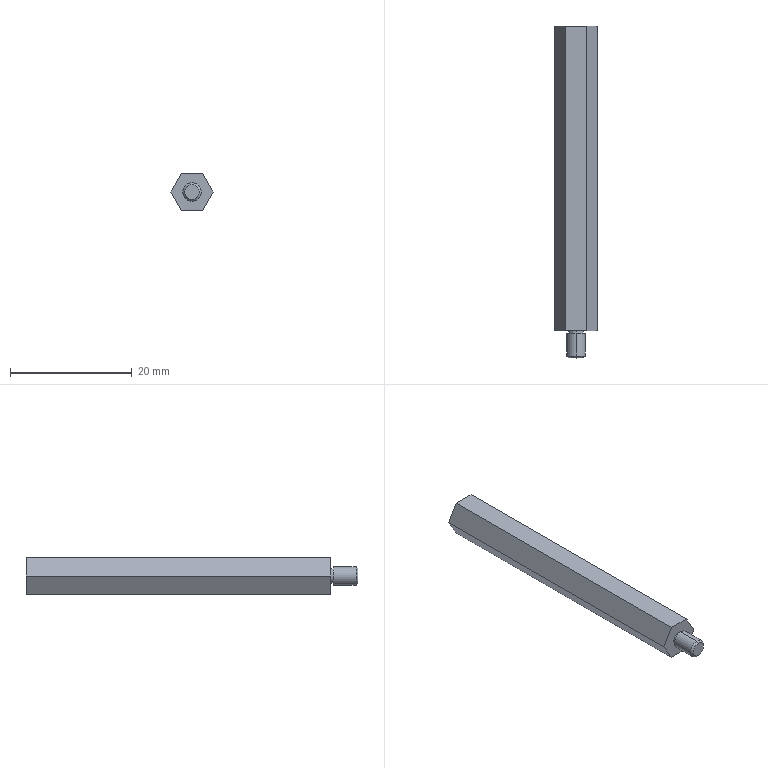Part | STEP file | 0230_017_LSBWRK6-50 | 1 solid | 22 faces | box 6.928 x 54.5 x 6 mm | volume 1554 mm3 | plane 10 | cone 6 | cylinder 6 | commonest cylinder face diameters 2.4 x2 2.5 x2 3 x2
STEP:
#1=CARTESIAN_POINT('',(0.,0.,0.));
#2=DIRECTION('',(0.,0.,1.));
#3=DIRECTION('',(1.,0.,0.));
#4=AXIS2_PLACEMENT_3D('',#1,#2,#3);
#5=CARTESIAN_POINT('',(0.,49.844,1.25));
#6=VERTEX_POINT('',#5);
#7=CARTESIAN_POINT('',(0.,50.,1.52));
#8=VERTEX_POINT('',#7);
#9=CARTESIAN_POINT('',(0.,49.844,1.25));
#10=DIRECTION('',(0.,0.5,0.866));
#11=VECTOR('',#10,1.);
#12=LINE('',#9,#11);
#13=CARTESIAN_POINT('',(0.,49.844,0.));
#14=DIRECTION('',(0.,1.,0.));
#15=DIRECTION('',(0.,0.,1.));
#16=AXIS2_PLACEMENT_3D('',#13,#14,#15);
#17=CONICAL_SURFACE('',#16,1.25,1.047);
#18=CARTESIAN_POINT('',(6.283,0.));
#19=DIRECTION('',(0.,1.));
#20=VECTOR('',#19,1.);
#21=LINE('',#18,#20);
#22=(GEOMETRIC_REPRESENTATION_CONTEXT(2)PARAMETRIC_REPRESENTATION_CONTEXT()REPRESENTATION_CONTEXT('',''));
#23=DEFINITIONAL_REPRESENTATION('',(#21),#22);
#24=PCURVE('',#17,#23);
#25=CARTESIAN_POINT('',(0.,49.844,0.));
#26=DIRECTION('',(0.,1.,0.));
#27=DIRECTION('',(0.,0.,1.));
#28=AXIS2_PLACEMENT_3D('',#25,#26,#27);
#29=CONICAL_SURFACE('',#28,1.25,1.047);
#30=CARTESIAN_POINT('',(0.,0.));
#31=DIRECTION('',(0.,1.));
#32=VECTOR('',#31,1.);
#33=LINE('',#30,#32);
#34=(GEOMETRIC_REPRESENTATION_CONTEXT(2)PARAMETRIC_REPRESENTATION_CONTEXT()REPRESENTATION_CONTEXT('',''));
#35=DEFINITIONAL_REPRESENTATION('',(#33),#34);
#36=PCURVE('',#29,#35);
#37=SURFACE_CURVE('',#12,(#24,#36),.PCURVE_S1.);
#38=EDGE_CURVE('',#6,#8,#37,.T.);
#39=ORIENTED_EDGE('',*,*,#38,.T.);
#40=CARTESIAN_POINT('',(0.,50.,-1.52));
#41=VERTEX_POINT('',#40);
#42=CARTESIAN_POINT('',(0.,50.,0.));
#43=DIRECTION('',(0.,-1.,0.));
#44=DIRECTION('',(1.,0.,0.));
#45=AXIS2_PLACEMENT_3D('',#42,#43,#44);
#46=CIRCLE('',#45,1.52);
#47=CARTESIAN_POINT('',(7.854,0.1559));
#48=DIRECTION('',(-1.,0.));
#49=VECTOR('',#48,1.);
#50=LINE('',#47,#49);
#51=(GEOMETRIC_REPRESENTATION_CONTEXT(2)PARAMETRIC_REPRESENTATION_CONTEXT()REPRESENTATION_CONTEXT('',''));
#52=DEFINITIONAL_REPRESENTATION('',(#50),#51);
#53=PCURVE('',#17,#52);
#54=CARTESIAN_POINT('',(3.464,50.,0.));
#55=DIRECTION('',(0.,-1.,0.));
#56=DIRECTION('',(1.,0.,0.));
#57=AXIS2_PLACEMENT_3D('',#54,#55,#56);
#58=PLANE('',#57);
#59=CARTESIAN_POINT('',(-3.464,0.));
#60=DIRECTION('',(1.,0.));
#61=AXIS2_PLACEMENT_2D('',#59,#60);
#62=CIRCLE('',#61,1.52);
#63=(GEOMETRIC_REPRESENTATION_CONTEXT(2)PARAMETRIC_REPRESENTATION_CONTEXT()REPRESENTATION_CONTEXT('',''));
#64=DEFINITIONAL_REPRESENTATION('',(#62),#63);
#65=PCURVE('',#58,#64);
#66=SURFACE_CURVE('',#46,(#53,#65),.PCURVE_S1.);
#67=EDGE_CURVE('',#8,#41,#66,.T.);
#68=ORIENTED_EDGE('',*,*,#67,.T.);
#69=CARTESIAN_POINT('',(0.,49.844,-1.25));
#70=VERTEX_POINT('',#69);
#71=CARTESIAN_POINT('',(0.,49.844,-1.25));
#72=DIRECTION('',(0.,0.5,-0.866));
#73=VECTOR('',#72,1.);
#74=LINE('',#71,#73);
#75=CARTESIAN_POINT('',(3.142,0.));
#76=DIRECTION('',(0.,1.));
#77=VECTOR('',#76,1.);
#78=LINE('',#75,#77);
#79=(GEOMETRIC_REPRESENTATION_CONTEXT(2)PARAMETRIC_REPRESENTATION_CONTEXT()REPRESENTATION_CONTEXT('',''));
#80=DEFINITIONAL_REPRESENTATION('',(#78),#79);
#81=PCURVE('',#17,#80);
#82=CARTESIAN_POINT('',(3.142,0.));
#83=DIRECTION('',(0.,1.));
#84=VECTOR('',#83,1.);
#85=LINE('',#82,#84);
#86=(GEOMETRIC_REPRESENTATION_CONTEXT(2)PARAMETRIC_REPRESENTATION_CONTEXT()REPRESENTATION_CONTEXT('',''));
#87=DEFINITIONAL_REPRESENTATION('',(#85),#86);
#88=PCURVE('',#29,#87);
#89=SURFACE_CURVE('',#74,(#81,#88),.PCURVE_S1.);
#90=EDGE_CURVE('',#70,#41,#89,.T.);
#91=ORIENTED_EDGE('',*,*,#90,.F.);
#92=CARTESIAN_POINT('',(0.,49.844,0.));
#93=DIRECTION('',(0.,1.,0.));
#94=DIRECTION('',(0.,0.,-1.));
#95=AXIS2_PLACEMENT_3D('',#92,#93,#94);
#96=CIRCLE('',#95,1.25);
#97=CARTESIAN_POINT('',(3.142,0.));
#98=DIRECTION('',(1.,0.));
#99=VECTOR('',#98,1.);
#100=LINE('',#97,#99);
#101=(GEOMETRIC_REPRESENTATION_CONTEXT(2)PARAMETRIC_REPRESENTATION_CONTEXT()REPRESENTATION_CONTEXT('',''));
#102=DEFINITIONAL_REPRESENTATION('',(#100),#101);
#103=PCURVE('',#17,#102);
#104=CARTESIAN_POINT('',(0.,50.,0.));
#105=DIRECTION('',(0.,1.,0.));
#106=DIRECTION('',(0.,0.,1.));
#107=AXIS2_PLACEMENT_3D('',#104,#105,#106);
#108=CYLINDRICAL_SURFACE('',#107,1.25);
#109=CARTESIAN_POINT('',(3.142,-0.1559));
#110=DIRECTION('',(1.,0.));
#111=VECTOR('',#110,1.);
#112=LINE('',#109,#111);
#113=(GEOMETRIC_REPRESENTATION_CONTEXT(2)PARAMETRIC_REPRESENTATION_CONTEXT()REPRESENTATION_CONTEXT('',''));
#114=DEFINITIONAL_REPRESENTATION('',(#112),#113);
#115=PCURVE('',#108,#114);
#116=SURFACE_CURVE('',#96,(#103,#115),.PCURVE_S1.);
#117=EDGE_CURVE('',#70,#6,#116,.T.);
#118=ORIENTED_EDGE('',*,*,#117,.T.);
#119=EDGE_LOOP('',(#39,#68,#91,#118));
#120=FACE_BOUND('',#119,.F.);
#121=ADVANCED_FACE('',(#120),#17,.F.);
#122=CARTESIAN_POINT('',(0.,-4.5,-1.193));
#123=VERTEX_POINT('',#122);
#124=CARTESIAN_POINT('',(0.,-4.5,1.193));
#125=VERTEX_POINT('',#124);
#126=CARTESIAN_POINT('',(0.,-4.5,0.));
#127=DIRECTION('',(0.,-1.,0.));
#128=DIRECTION('',(0.,0.,-1.));
#129=AXIS2_PLACEMENT_3D('',#126,#127,#128);
#130=CIRCLE('',#129,1.193);
#131=CARTESIAN_POINT('',(0.,-4.193,0.));
#132=DIRECTION('',(0.,1.,0.));
#133=DIRECTION('',(0.,0.,1.));
#134=AXIS2_PLACEMENT_3D('',#131,#132,#133);
#135=CONICAL_SURFACE('',#134,1.5,0.7854);
#136=CARTESIAN_POINT('',(3.142,-0.3065));
#137=DIRECTION('',(-1.,0.));
#138=VECTOR('',#137,1.);
#139=LINE('',#136,#138);
#140=(GEOMETRIC_REPRESENTATION_CONTEXT(2)PARAMETRIC_REPRESENTATION_CONTEXT()REPRESENTATION_CONTEXT('',''));
#141=DEFINITIONAL_REPRESENTATION('',(#139),#140);
#142=PCURVE('',#135,#141);
#143=CARTESIAN_POINT('',(1.5,-4.5,0.));
#144=DIRECTION('',(0.,-1.,0.));
#145=DIRECTION('',(0.,0.,-1.));
#146=AXIS2_PLACEMENT_3D('',#143,#144,#145);
#147=PLANE('',#146);
#148=CARTESIAN_POINT('',(0.,-1.5));
#149=DIRECTION('',(1.,0.));
#150=AXIS2_PLACEMENT_2D('',#148,#149);
#151=CIRCLE('',#150,1.193);
#152=(GEOMETRIC_REPRESENTATION_CONTEXT(2)PARAMETRIC_REPRESENTATION_CONTEXT()REPRESENTATION_CONTEXT('',''));
#153=DEFINITIONAL_REPRESENTATION('',(#151),#152);
#154=PCURVE('',#147,#153);
#155=SURFACE_CURVE('',#130,(#142,#154),.PCURVE_S1.);
#156=EDGE_CURVE('',#123,#125,#155,.T.);
#157=ORIENTED_EDGE('',*,*,#156,.F.);
#158=CARTESIAN_POINT('',(0.,-4.193,-1.5));
#159=VERTEX_POINT('',#158);
#160=CARTESIAN_POINT('',(0.,-4.193,-1.5));
#161=DIRECTION('',(0.,0.7071,-0.7071));
#162=VECTOR('',#161,1.);
#163=LINE('',#160,#162);
#164=CARTESIAN_POINT('',(3.142,0.));
#165=DIRECTION('',(0.,1.));
#166=VECTOR('',#165,1.);
#167=LINE('',#164,#166);
#168=(GEOMETRIC_REPRESENTATION_CONTEXT(2)PARAMETRIC_REPRESENTATION_CONTEXT()REPRESENTATION_CONTEXT('',''));
#169=DEFINITIONAL_REPRESENTATION('',(#167),#168);
#170=PCURVE('',#135,#169);
#171=CARTESIAN_POINT('',(0.,-4.193,0.));
#172=DIRECTION('',(0.,1.,0.));
#173=DIRECTION('',(0.,0.,1.));
#174=AXIS2_PLACEMENT_3D('',#171,#172,#173);
#175=CONICAL_SURFACE('',#174,1.5,0.7854);
#176=CARTESIAN_POINT('',(3.142,0.));
#177=DIRECTION('',(0.,1.));
#178=VECTOR('',#177,1.);
#179=LINE('',#176,#178);
#180=(GEOMETRIC_REPRESENTATION_CONTEXT(2)PARAMETRIC_REPRESENTATION_CONTEXT()REPRESENTATION_CONTEXT('',''));
#181=DEFINITIONAL_REPRESENTATION('',(#179),#180);
#182=PCURVE('',#175,#181);
#183=SURFACE_CURVE('',#163,(#170,#182),.PCURVE_S1.);
#184=EDGE_CURVE('',#123,#159,#183,.T.);
#185=ORIENTED_EDGE('',*,*,#184,.T.);
#186=CARTESIAN_POINT('',(0.,-4.193,1.5));
#187=VERTEX_POINT('',#186);
#188=CARTESIAN_POINT('',(0.,-4.193,0.));
#189=DIRECTION('',(0.,1.,0.));
#190=DIRECTION('',(0.,0.,-1.));
#191=AXIS2_PLACEMENT_3D('',#188,#189,#190);
#192=CIRCLE('',#191,1.5);
#193=CARTESIAN_POINT('',(-3.142,0.));
#194=DIRECTION('',(1.,0.));
#195=VECTOR('',#194,1.);
#196=LINE('',#193,#195);
#197=(GEOMETRIC_REPRESENTATION_CONTEXT(2)PARAMETRIC_REPRESENTATION_CONTEXT()REPRESENTATION_CONTEXT('',''));
#198=DEFINITIONAL_REPRESENTATION('',(#196),#197);
#199=PCURVE('',#135,#198);
#200=CARTESIAN_POINT('',(0.,-4.5,0.));
#201=DIRECTION('',(0.,1.,0.));
#202=DIRECTION('',(0.,0.,1.));
#203=AXIS2_PLACEMENT_3D('',#200,#201,#202);
#204=CYLINDRICAL_SURFACE('',#203,1.5);
#205=CARTESIAN_POINT('',(-3.142,0.3065));
#206=DIRECTION('',(1.,0.));
#207=VECTOR('',#206,1.);
#208=LINE('',#205,#207);
#209=(GEOMETRIC_REPRESENTATION_CONTEXT(2)PARAMETRIC_REPRESENTATION_CONTEXT()REPRESENTATION_CONTEXT('',''));
#210=DEFINITIONAL_REPRESENTATION('',(#208),#209);
#211=PCURVE('',#204,#210);
#212=SURFACE_CURVE('',#192,(#199,#211),.PCURVE_S1.);
#213=EDGE_CURVE('',#187,#159,#212,.T.);
#214=ORIENTED_EDGE('',*,*,#213,.F.);
#215=CARTESIAN_POINT('',(0.,-4.193,1.5));
#216=DIRECTION('',(0.,0.7071,0.7071));
#217=VECTOR('',#216,1.);
#218=LINE('',#215,#217);
#219=CARTESIAN_POINT('',(0.,0.));
#220=DIRECTION('',(0.,1.));
#221=VECTOR('',#220,1.);
#222=LINE('',#219,#221);
#223=(GEOMETRIC_REPRESENTATION_CONTEXT(2)PARAMETRIC_REPRESENTATION_CONTEXT()REPRESENTATION_CONTEXT('',''));
#224=DEFINITIONAL_REPRESENTATION('',(#222),#223);
#225=PCURVE('',#135,#224);
#226=CARTESIAN_POINT('',(6.283,0.));
#227=DIRECTION('',(0.,1.));
#228=VECTOR('',#227,1.);
#229=LINE('',#226,#228);
#230=(GEOMETRIC_REPRESENTATION_CONTEXT(2)PARAMETRIC_REPRESENTATION_CONTEXT()REPRESENTATION_CONTEXT('',''));
#231=DEFINITIONAL_REPRESENTATION('',(#229),#230);
#232=PCURVE('',#175,#231);
#233=SURFACE_CURVE('',#218,(#225,#232),.PCURVE_S1.);
#234=EDGE_CURVE('',#125,#187,#233,.T.);
#235=ORIENTED_EDGE('',*,*,#234,.F.);
#236=EDGE_LOOP('',(#157,#185,#214,#235));
#237=FACE_BOUND('',#236,.T.);
#238=ADVANCED_FACE('',(#237),#135,.T.);
#239=CARTESIAN_POINT('',(0.,43.2,1.25));
#240=VERTEX_POINT('',#239);
#241=CARTESIAN_POINT('',(0.,50.,1.25));
#242=DIRECTION('',(0.,1.,0.));
#243=VECTOR('',#242,1.);
#244=LINE('',#241,#243);
#245=CARTESIAN_POINT('',(6.283,0.));
#246=DIRECTION('',(0.,1.));
#247=VECTOR('',#246,1.);
#248=LINE('',#245,#247);
#249=(GEOMETRIC_REPRESENTATION_CONTEXT(2)PARAMETRIC_REPRESENTATION_CONTEXT()REPRESENTATION_CONTEXT('',''));
#250=DEFINITIONAL_REPRESENTATION('',(#248),#249);
#251=PCURVE('',#108,#250);
#252=CARTESIAN_POINT('',(0.,50.,0.));
#253=DIRECTION('',(0.,1.,0.));
#254=DIRECTION('',(0.,0.,1.));
#255=AXIS2_PLACEMENT_3D('',#252,#253,#254);
#256=CYLINDRICAL_SURFACE('',#255,1.25);
#257=CARTESIAN_POINT('',(0.,0.));
#258=DIRECTION('',(0.,1.));
#259=VECTOR('',#258,1.);
#260=LINE('',#257,#259);
#261=(GEOMETRIC_REPRESENTATION_CONTEXT(2)PARAMETRIC_REPRESENTATION_CONTEXT()REPRESENTATION_CONTEXT('',''));
#262=DEFINITIONAL_REPRESENTATION('',(#260),#261);
#263=PCURVE('',#256,#262);
#264=SURFACE_CURVE('',#244,(#251,#263),.PCURVE_S1.);
#265=EDGE_CURVE('',#240,#6,#264,.T.);
#266=ORIENTED_EDGE('',*,*,#265,.T.);
#267=ORIENTED_EDGE('',*,*,#117,.F.);
#268=CARTESIAN_POINT('',(0.,43.2,-1.25));
#269=VERTEX_POINT('',#268);
#270=CARTESIAN_POINT('',(0.,50.,-1.25));
#271=DIRECTION('',(0.,1.,0.));
#272=VECTOR('',#271,1.);
#273=LINE('',#270,#272);
#274=CARTESIAN_POINT('',(3.142,0.));
#275=DIRECTION('',(0.,1.));
#276=VECTOR('',#275,1.);
#277=LINE('',#274,#276);
#278=(GEOMETRIC_REPRESENTATION_CONTEXT(2)PARAMETRIC_REPRESENTATION_CONTEXT()REPRESENTATION_CONTEXT('',''));
#279=DEFINITIONAL_REPRESENTATION('',(#277),#278);
#280=PCURVE('',#108,#279);
#281=CARTESIAN_POINT('',(3.142,0.));
#282=DIRECTION('',(0.,1.));
#283=VECTOR('',#282,1.);
#284=LINE('',#281,#283);
#285=(GEOMETRIC_REPRESENTATION_CONTEXT(2)PARAMETRIC_REPRESENTATION_CONTEXT()REPRESENTATION_CONTEXT('',''));
#286=DEFINITIONAL_REPRESENTATION('',(#284),#285);
#287=PCURVE('',#256,#286);
#288=SURFACE_CURVE('',#273,(#280,#287),.PCURVE_S1.);
#289=EDGE_CURVE('',#269,#70,#288,.T.);
#290=ORIENTED_EDGE('',*,*,#289,.F.);
#291=CARTESIAN_POINT('',(0.,43.2,0.));
#292=DIRECTION('',(0.,1.,0.));
#293=DIRECTION('',(0.,0.,1.));
#294=AXIS2_PLACEMENT_3D('',#291,#292,#293);
#295=CIRCLE('',#294,1.25);
#296=CARTESIAN_POINT('',(0.,-6.8));
#297=DIRECTION('',(1.,0.));
#298=VECTOR('',#297,1.);
#299=LINE('',#296,#298);
#300=(GEOMETRIC_REPRESENTATION_CONTEXT(2)PARAMETRIC_REPRESENTATION_CONTEXT()REPRESENTATION_CONTEXT('',''));
#301=DEFINITIONAL_REPRESENTATION('',(#299),#300);
#302=PCURVE('',#108,#301);
#303=CARTESIAN_POINT('',(0.,43.2,0.));
#304=DIRECTION('',(0.,1.,0.));
#305=DIRECTION('',(0.,0.,1.));
#306=AXIS2_PLACEMENT_3D('',#303,#304,#305);
#307=CONICAL_SURFACE('',#306,1.25,1.03);
#308=CARTESIAN_POINT('',(0.,0.));
#309=DIRECTION('',(1.,0.));
#310=VECTOR('',#309,1.);
#311=LINE('',#308,#310);
#312=(GEOMETRIC_REPRESENTATION_CONTEXT(2)PARAMETRIC_REPRESENTATION_CONTEXT()REPRESENTATION_CONTEXT('',''));
#313=DEFINITIONAL_REPRESENTATION('',(#311),#312);
#314=PCURVE('',#307,#313);
#315=SURFACE_CURVE('',#295,(#302,#314),.PCURVE_S1.);
#316=EDGE_CURVE('',#269,#240,#315,.T.);
#317=ORIENTED_EDGE('',*,*,#316,.T.);
#318=EDGE_LOOP('',(#266,#267,#290,#317));
#319=FACE_BOUND('',#318,.F.);
#320=ADVANCED_FACE('',(#319),#108,.F.);
#321=ORIENTED_EDGE('',*,*,#316,.F.);
#322=CARTESIAN_POINT('',(0.,42.449,0.));
#323=VERTEX_POINT('',#322);
#324=CARTESIAN_POINT('',(0.,43.2,-1.25));
#325=DIRECTION('',(0.,0.515,-0.8572));
#326=VECTOR('',#325,1.);
#327=LINE('',#324,#326);
#328=CARTESIAN_POINT('',(3.142,0.));
#329=DIRECTION('',(0.,1.));
#330=VECTOR('',#329,1.);
#331=LINE('',#328,#330);
#332=(GEOMETRIC_REPRESENTATION_CONTEXT(2)PARAMETRIC_REPRESENTATION_CONTEXT()REPRESENTATION_CONTEXT('',''));
#333=DEFINITIONAL_REPRESENTATION('',(#331),#332);
#334=PCURVE('',#307,#333);
#335=CARTESIAN_POINT('',(0.,43.2,0.));
#336=DIRECTION('',(0.,1.,0.));
#337=DIRECTION('',(0.,0.,1.));
#338=AXIS2_PLACEMENT_3D('',#335,#336,#337);
#339=CONICAL_SURFACE('',#338,1.25,1.03);
#340=CARTESIAN_POINT('',(3.142,0.));
#341=DIRECTION('',(0.,1.));
#342=VECTOR('',#341,1.);
#343=LINE('',#340,#342);
#344=(GEOMETRIC_REPRESENTATION_CONTEXT(2)PARAMETRIC_REPRESENTATION_CONTEXT()REPRESENTATION_CONTEXT('',''));
#345=DEFINITIONAL_REPRESENTATION('',(#343),#344);
#346=PCURVE('',#339,#345);
#347=SURFACE_CURVE('',#327,(#334,#346),.PCURVE_S1.);
#348=EDGE_CURVE('',#323,#269,#347,.T.);
#349=ORIENTED_EDGE('',*,*,#348,.F.);
#350=CARTESIAN_POINT('',(0.,43.2,1.25));
#351=DIRECTION('',(0.,0.515,0.8572));
#352=VECTOR('',#351,1.);
#353=LINE('',#350,#352);
#354=CARTESIAN_POINT('',(6.283,0.));
#355=DIRECTION('',(0.,1.));
#356=VECTOR('',#355,1.);
#357=LINE('',#354,#356);
#358=(GEOMETRIC_REPRESENTATION_CONTEXT(2)PARAMETRIC_REPRESENTATION_CONTEXT()REPRESENTATION_CONTEXT('',''));
#359=DEFINITIONAL_REPRESENTATION('',(#357),#358);
#360=PCURVE('',#307,#359);
#361=CARTESIAN_POINT('',(0.,0.));
#362=DIRECTION('',(0.,1.));
#363=VECTOR('',#362,1.);
#364=LINE('',#361,#363);
#365=(GEOMETRIC_REPRESENTATION_CONTEXT(2)PARAMETRIC_REPRESENTATION_CONTEXT()REPRESENTATION_CONTEXT('',''));
#366=DEFINITIONAL_REPRESENTATION('',(#364),#365);
#367=PCURVE('',#339,#366);
#368=SURFACE_CURVE('',#353,(#360,#367),.PCURVE_S1.);
#369=EDGE_CURVE('',#323,#240,#368,.T.);
#370=ORIENTED_EDGE('',*,*,#369,.T.);
#371=EDGE_LOOP('',(#321,#349,#370));
#372=FACE_BOUND('',#371,.F.);
#373=ADVANCED_FACE('',(#372),#307,.F.);
#374=CARTESIAN_POINT('',(0.,-0.45,1.2));
#375=VERTEX_POINT('',#374);
#376=CARTESIAN_POINT('',(0.,-0.45,-1.2));
#377=VERTEX_POINT('',#376);
#378=CARTESIAN_POINT('',(0.,-0.45,0.));
#379=DIRECTION('',(0.,1.,0.));
#380=DIRECTION('',(0.,0.,1.));
#381=AXIS2_PLACEMENT_3D('',#378,#379,#380);
#382=CIRCLE('',#381,1.2);
#383=CARTESIAN_POINT('',(0.,-4.5,0.));
#384=DIRECTION('',(0.,1.,0.));
#385=DIRECTION('',(0.,0.,1.));
#386=AXIS2_PLACEMENT_3D('',#383,#384,#385);
#387=CYLINDRICAL_SURFACE('',#386,1.2);
#388=CARTESIAN_POINT('',(0.,4.05));
#389=DIRECTION('',(1.,0.));
#390=VECTOR('',#389,1.);
#391=LINE('',#388,#390);
#392=(GEOMETRIC_REPRESENTATION_CONTEXT(2)PARAMETRIC_REPRESENTATION_CONTEXT()REPRESENTATION_CONTEXT('',''));
#393=DEFINITIONAL_REPRESENTATION('',(#391),#392);
#394=PCURVE('',#387,#393);
#395=CARTESIAN_POINT('',(1.2,-0.45,0.));
#396=DIRECTION('',(0.,1.,0.));
#397=DIRECTION('',(0.,0.,1.));
#398=AXIS2_PLACEMENT_3D('',#395,#396,#397);
#399=PLANE('',#398);
#400=CARTESIAN_POINT('',(0.,-1.2));
#401=DIRECTION('',(1.,0.));
#402=AXIS2_PLACEMENT_2D('',#400,#401);
#403=CIRCLE('',#402,1.2);
#404=(GEOMETRIC_REPRESENTATION_CONTEXT(2)PARAMETRIC_REPRESENTATION_CONTEXT()REPRESENTATION_CONTEXT('',''));
#405=DEFINITIONAL_REPRESENTATION('',(#403),#404);
#406=PCURVE('',#399,#405);
#407=SURFACE_CURVE('',#382,(#394,#406),.PCURVE_S1.);
#408=EDGE_CURVE('',#375,#377,#407,.T.);
#409=ORIENTED_EDGE('',*,*,#408,.T.);
#410=CARTESIAN_POINT('',(0.,0.,-1.2));
#411=VERTEX_POINT('',#410);
#412=CARTESIAN_POINT('',(0.,-4.5,-1.2));
#413=DIRECTION('',(0.,1.,0.));
#414=VECTOR('',#413,1.);
#415=LINE('',#412,#414);
#416=CARTESIAN_POINT('',(3.142,0.));
#417=DIRECTION('',(0.,1.));
#418=VECTOR('',#417,1.);
#419=LINE('',#416,#418);
#420=(GEOMETRIC_REPRESENTATION_CONTEXT(2)PARAMETRIC_REPRESENTATION_CONTEXT()REPRESENTATION_CONTEXT('',''));
#421=DEFINITIONAL_REPRESENTATION('',(#419),#420);
#422=PCURVE('',#387,#421);
#423=CARTESIAN_POINT('',(0.,-4.5,0.));
#424=DIRECTION('',(0.,1.,0.));
#425=DIRECTION('',(0.,0.,1.));
#426=AXIS2_PLACEMENT_3D('',#423,#424,#425);
#427=CYLINDRICAL_SURFACE('',#426,1.2);
#428=CARTESIAN_POINT('',(3.142,0.));
#429=DIRECTION('',(0.,1.));
#430=VECTOR('',#429,1.);
#431=LINE('',#428,#430);
#432=(GEOMETRIC_REPRESENTATION_CONTEXT(2)PARAMETRIC_REPRESENTATION_CONTEXT()REPRESENTATION_CONTEXT('',''));
#433=DEFINITIONAL_REPRESENTATION('',(#431),#432);
#434=PCURVE('',#427,#433);
#435=SURFACE_CURVE('',#415,(#422,#434),.PCURVE_S1.);
#436=EDGE_CURVE('',#377,#411,#435,.T.);
#437=ORIENTED_EDGE('',*,*,#436,.T.);
#438=CARTESIAN_POINT('',(0.,0.,1.2));
#439=VERTEX_POINT('',#438);
#440=CARTESIAN_POINT('',(0.,0.,0.));
#441=DIRECTION('',(0.,-1.,0.));
#442=DIRECTION('',(1.,0.,0.));
#443=AXIS2_PLACEMENT_3D('',#440,#441,#442);
#444=CIRCLE('',#443,1.2);
#445=CARTESIAN_POINT('',(7.854,4.5));
#446=DIRECTION('',(-1.,0.));
#447=VECTOR('',#446,1.);
#448=LINE('',#445,#447);
#449=(GEOMETRIC_REPRESENTATION_CONTEXT(2)PARAMETRIC_REPRESENTATION_CONTEXT()REPRESENTATION_CONTEXT('',''));
#450=DEFINITIONAL_REPRESENTATION('',(#448),#449);
#451=PCURVE('',#387,#450);
#452=CARTESIAN_POINT('',(3.464,0.,0.));
#453=DIRECTION('',(0.,-1.,0.));
#454=DIRECTION('',(1.,0.,0.));
#455=AXIS2_PLACEMENT_3D('',#452,#453,#454);
#456=PLANE('',#455);
#457=CARTESIAN_POINT('',(-3.464,0.));
#458=DIRECTION('',(1.,0.));
#459=AXIS2_PLACEMENT_2D('',#457,#458);
#460=CIRCLE('',#459,1.2);
#461=(GEOMETRIC_REPRESENTATION_CONTEXT(2)PARAMETRIC_REPRESENTATION_CONTEXT()REPRESENTATION_CONTEXT('',''));
#462=DEFINITIONAL_REPRESENTATION('',(#460),#461);
#463=PCURVE('',#456,#462);
#464=SURFACE_CURVE('',#444,(#451,#463),.PCURVE_S1.);
#465=EDGE_CURVE('',#411,#439,#464,.T.);
#466=ORIENTED_EDGE('',*,*,#465,.T.);
#467=CARTESIAN_POINT('',(0.,-4.5,1.2));
#468=DIRECTION('',(0.,1.,0.));
#469=VECTOR('',#468,1.);
#470=LINE('',#467,#469);
#471=CARTESIAN_POINT('',(0.,0.));
#472=DIRECTION('',(0.,1.));
#473=VECTOR('',#472,1.);
#474=LINE('',#471,#473);
#475=(GEOMETRIC_REPRESENTATION_CONTEXT(2)PARAMETRIC_REPRESENTATION_CONTEXT()REPRESENTATION_CONTEXT('',''));
#476=DEFINITIONAL_REPRESENTATION('',(#474),#475);
#477=PCURVE('',#387,#476);
#478=CARTESIAN_POINT('',(6.283,0.));
#479=DIRECTION('',(0.,1.));
#480=VECTOR('',#479,1.);
#481=LINE('',#478,#480);
#482=(GEOMETRIC_REPRESENTATION_CONTEXT(2)PARAMETRIC_REPRESENTATION_CONTEXT()REPRESENTATION_CONTEXT('',''));
#483=DEFINITIONAL_REPRESENTATION('',(#481),#482);
#484=PCURVE('',#427,#483);
#485=SURFACE_CURVE('',#470,(#477,#484),.PCURVE_S1.);
#486=EDGE_CURVE('',#375,#439,#485,.T.);
#487=ORIENTED_EDGE('',*,*,#486,.F.);
#488=EDGE_LOOP('',(#409,#437,#466,#487));
#489=FACE_BOUND('',#488,.T.);
#490=ADVANCED_FACE('',(#489),#387,.T.);
#491=ORIENTED_EDGE('',*,*,#213,.T.);
#492=CARTESIAN_POINT('',(0.,-0.45,-1.5));
#493=VERTEX_POINT('',#492);
#494=CARTESIAN_POINT('',(0.,-4.5,-1.5));
#495=DIRECTION('',(0.,1.,0.));
#496=VECTOR('',#495,1.);
#497=LINE('',#494,#496);
#498=CARTESIAN_POINT('',(3.142,0.));
#499=DIRECTION('',(0.,1.));
#500=VECTOR('',#499,1.);
#501=LINE('',#498,#500);
#502=(GEOMETRIC_REPRESENTATION_CONTEXT(2)PARAMETRIC_REPRESENTATION_CONTEXT()REPRESENTATION_CONTEXT('',''));
#503=DEFINITIONAL_REPRESENTATION('',(#501),#502);
#504=PCURVE('',#204,#503);
#505=CARTESIAN_POINT('',(0.,-4.5,0.));
#506=DIRECTION('',(0.,1.,0.));
#507=DIRECTION('',(0.,0.,1.));
#508=AXIS2_PLACEMENT_3D('',#505,#506,#507);
#509=CYLINDRICAL_SURFACE('',#508,1.5);
#510=CARTESIAN_POINT('',(3.142,0.));
#511=DIRECTION('',(0.,1.));
#512=VECTOR('',#511,1.);
#513=LINE('',#510,#512);
#514=(GEOMETRIC_REPRESENTATION_CONTEXT(2)PARAMETRIC_REPRESENTATION_CONTEXT()REPRESENTATION_CONTEXT('',''));
#515=DEFINITIONAL_REPRESENTATION('',(#513),#514);
#516=PCURVE('',#509,#515);
#517=SURFACE_CURVE('',#497,(#504,#516),.PCURVE_S1.);
#518=EDGE_CURVE('',#159,#493,#517,.T.);
#519=ORIENTED_EDGE('',*,*,#518,.T.);
#520=CARTESIAN_POINT('',(0.,-0.45,1.5));
#521=VERTEX_POINT('',#520);
#522=CARTESIAN_POINT('',(0.,-0.45,0.));
#523=DIRECTION('',(0.,1.,0.));
#524=DIRECTION('',(0.,0.,1.));
#525=AXIS2_PLACEMENT_3D('',#522,#523,#524);
#526=CIRCLE('',#525,1.5);
#527=CARTESIAN_POINT('',(0.,4.05));
#528=DIRECTION('',(1.,0.));
#529=VECTOR('',#528,1.);
#530=LINE('',#527,#529);
#531=(GEOMETRIC_REPRESENTATION_CONTEXT(2)PARAMETRIC_REPRESENTATION_CONTEXT()REPRESENTATION_CONTEXT('',''));
#532=DEFINITIONAL_REPRESENTATION('',(#530),#531);
#533=PCURVE('',#204,#532);
#534=CARTESIAN_POINT('',(0.,-1.2));
#535=DIRECTION('',(1.,0.));
#536=AXIS2_PLACEMENT_2D('',#534,#535);
#537=CIRCLE('',#536,1.5);
#538=(GEOMETRIC_REPRESENTATION_CONTEXT(2)PARAMETRIC_REPRESENTATION_CONTEXT()REPRESENTATION_CONTEXT('',''));
#539=DEFINITIONAL_REPRESENTATION('',(#537),#538);
#540=PCURVE('',#399,#539);
#541=SURFACE_CURVE('',#526,(#533,#540),.PCURVE_S1.);
#542=EDGE_CURVE('',#521,#493,#541,.T.);
#543=ORIENTED_EDGE('',*,*,#542,.F.);
#544=CARTESIAN_POINT('',(0.,-4.5,1.5));
#545=DIRECTION('',(0.,1.,0.));
#546=VECTOR('',#545,1.);
#547=LINE('',#544,#546);
#548=CARTESIAN_POINT('',(0.,0.));
#549=DIRECTION('',(0.,1.));
#550=VECTOR('',#549,1.);
#551=LINE('',#548,#550);
#552=(GEOMETRIC_REPRESENTATION_CONTEXT(2)PARAMETRIC_REPRESENTATION_CONTEXT()REPRESENTATION_CONTEXT('',''));
#553=DEFINITIONAL_REPRESENTATION('',(#551),#552);
#554=PCURVE('',#204,#553);
#555=CARTESIAN_POINT('',(6.283,0.));
#556=DIRECTION('',(0.,1.));
#557=VECTOR('',#556,1.);
#558=LINE('',#555,#557);
#559=(GEOMETRIC_REPRESENTATION_CONTEXT(2)PARAMETRIC_REPRESENTATION_CONTEXT()REPRESENTATION_CONTEXT('',''));
#560=DEFINITIONAL_REPRESENTATION('',(#558),#559);
#561=PCURVE('',#509,#560);
#562=SURFACE_CURVE('',#547,(#554,#561),.PCURVE_S1.);
#563=EDGE_CURVE('',#187,#521,#562,.T.);
#564=ORIENTED_EDGE('',*,*,#563,.F.);
#565=EDGE_LOOP('',(#491,#519,#543,#564));
#566=FACE_BOUND('',#565,.T.);
#567=ADVANCED_FACE('',(#566),#204,.T.);
#568=CARTESIAN_POINT('',(1.732,0.,-3.));
#569=VERTEX_POINT('',#568);
#570=CARTESIAN_POINT('',(3.464,0.,0.));
#571=VERTEX_POINT('',#570);
#572=CARTESIAN_POINT('',(1.732,0.,-3.));
#573=DIRECTION('',(0.5,0.,0.866));
#574=VECTOR('',#573,1.);
#575=LINE('',#572,#574);
#576=CARTESIAN_POINT('',(1.732,50.,-3.));
#577=DIRECTION('',(0.866,0.,-0.5));
#578=DIRECTION('',(-0.5,0.,-0.866));
#579=AXIS2_PLACEMENT_3D('',#576,#577,#578);
#580=PLANE('',#579);
#581=CARTESIAN_POINT('',(0.,-50.));
#582=DIRECTION('',(-1.,0.));
#583=VECTOR('',#582,1.);
#584=LINE('',#581,#583);
#585=(GEOMETRIC_REPRESENTATION_CONTEXT(2)PARAMETRIC_REPRESENTATION_CONTEXT()REPRESENTATION_CONTEXT('',''));
#586=DEFINITIONAL_REPRESENTATION('',(#584),#585);
#587=PCURVE('',#580,#586);
#588=CARTESIAN_POINT('',(-1.732,-3.));
#589=DIRECTION('',(0.5,0.866));
#590=VECTOR('',#589,1.);
#591=LINE('',#588,#590);
#592=(GEOMETRIC_REPRESENTATION_CONTEXT(2)PARAMETRIC_REPRESENTATION_CONTEXT()REPRESENTATION_CONTEXT('',''));
#593=DEFINITIONAL_REPRESENTATION('',(#591),#592);
#594=PCURVE('',#456,#593);
#595=SURFACE_CURVE('',#575,(#587,#594),.PCURVE_S1.);
#596=EDGE_CURVE('',#569,#571,#595,.T.);
#597=ORIENTED_EDGE('',*,*,#596,.F.);
#598=CARTESIAN_POINT('',(1.732,50.,-3.));
#599=VERTEX_POINT('',#598);
#600=CARTESIAN_POINT('',(1.732,50.,-3.));
#601=DIRECTION('',(0.,-1.,0.));
#602=VECTOR('',#601,1.);
#603=LINE('',#600,#602);
#604=CARTESIAN_POINT('',(0.,0.));
#605=DIRECTION('',(0.,-1.));
#606=VECTOR('',#605,1.);
#607=LINE('',#604,#606);
#608=(GEOMETRIC_REPRESENTATION_CONTEXT(2)PARAMETRIC_REPRESENTATION_CONTEXT()REPRESENTATION_CONTEXT('',''));
#609=DEFINITIONAL_REPRESENTATION('',(#607),#608);
#610=PCURVE('',#580,#609);
#611=CARTESIAN_POINT('',(-1.732,50.,-3.));
#612=DIRECTION('',(0.,0.,-1.));
#613=DIRECTION('',(-1.,0.,0.));
#614=AXIS2_PLACEMENT_3D('',#611,#612,#613);
#615=PLANE('',#614);
#616=CARTESIAN_POINT('',(-3.464,0.));
#617=DIRECTION('',(0.,-1.));
#618=VECTOR('',#617,1.);
#619=LINE('',#616,#618);
#620=(GEOMETRIC_REPRESENTATION_CONTEXT(2)PARAMETRIC_REPRESENTATION_CONTEXT()REPRESENTATION_CONTEXT('',''));
#621=DEFINITIONAL_REPRESENTATION('',(#619),#620);
#622=PCURVE('',#615,#621);
#623=SURFACE_CURVE('',#603,(#610,#622),.PCURVE_S1.);
#624=EDGE_CURVE('',#599,#569,#623,.T.);
#625=ORIENTED_EDGE('',*,*,#624,.F.);
#626=CARTESIAN_POINT('',(3.464,50.,0.));
#627=VERTEX_POINT('',#626);
#628=CARTESIAN_POINT('',(1.732,50.,-3.));
#629=DIRECTION('',(0.5,0.,0.866));
#630=VECTOR('',#629,1.);
#631=LINE('',#628,#630);
#632=CARTESIAN_POINT('',(0.,0.));
#633=DIRECTION('',(-1.,0.));
#634=VECTOR('',#633,1.);
#635=LINE('',#632,#634);
#636=(GEOMETRIC_REPRESENTATION_CONTEXT(2)PARAMETRIC_REPRESENTATION_CONTEXT()REPRESENTATION_CONTEXT('',''));
#637=DEFINITIONAL_REPRESENTATION('',(#635),#636);
#638=PCURVE('',#580,#637);
#639=CARTESIAN_POINT('',(-1.732,-3.));
#640=DIRECTION('',(0.5,0.866));
#641=VECTOR('',#640,1.);
#642=LINE('',#639,#641);
#643=(GEOMETRIC_REPRESENTATION_CONTEXT(2)PARAMETRIC_REPRESENTATION_CONTEXT()REPRESENTATION_CONTEXT('',''));
#644=DEFINITIONAL_REPRESENTATION('',(#642),#643);
#645=PCURVE('',#58,#644);
#646=SURFACE_CURVE('',#631,(#638,#645),.PCURVE_S1.);
#647=EDGE_CURVE('',#599,#627,#646,.T.);
#648=ORIENTED_EDGE('',*,*,#647,.T.);
#649=CARTESIAN_POINT('',(3.464,50.,0.));
#650=DIRECTION('',(0.,-1.,0.));
#651=VECTOR('',#650,1.);
#652=LINE('',#649,#651);
#653=CARTESIAN_POINT('',(-3.464,0.));
#654=DIRECTION('',(0.,-1.));
#655=VECTOR('',#654,1.);
#656=LINE('',#653,#655);
#657=(GEOMETRIC_REPRESENTATION_CONTEXT(2)PARAMETRIC_REPRESENTATION_CONTEXT()REPRESENTATION_CONTEXT('',''));
#658=DEFINITIONAL_REPRESENTATION('',(#656),#657);
#659=PCURVE('',#580,#658);
#660=CARTESIAN_POINT('',(3.464,50.,0.));
#661=DIRECTION('',(0.866,0.,0.5));
#662=DIRECTION('',(0.5,0.,-0.866));
#663=AXIS2_PLACEMENT_3D('',#660,#661,#662);
#664=PLANE('',#663);
#665=CARTESIAN_POINT('',(0.,0.));
#666=DIRECTION('',(0.,-1.));
#667=VECTOR('',#666,1.);
#668=LINE('',#665,#667);
#669=(GEOMETRIC_REPRESENTATION_CONTEXT(2)PARAMETRIC_REPRESENTATION_CONTEXT()REPRESENTATION_CONTEXT('',''));
#670=DEFINITIONAL_REPRESENTATION('',(#668),#669);
#671=PCURVE('',#664,#670);
#672=SURFACE_CURVE('',#652,(#659,#671),.PCURVE_S1.);
#673=EDGE_CURVE('',#627,#571,#672,.T.);
#674=ORIENTED_EDGE('',*,*,#673,.T.);
#675=EDGE_LOOP('',(#597,#625,#648,#674));
#676=FACE_BOUND('',#675,.T.);
#677=ADVANCED_FACE('',(#676),#580,.T.);
#678=CARTESIAN_POINT('',(-1.732,0.,-3.));
#679=VERTEX_POINT('',#678);
#680=CARTESIAN_POINT('',(-1.732,0.,-3.));
#681=DIRECTION('',(1.,0.,0.));
#682=VECTOR('',#681,1.);
#683=LINE('',#680,#682);
#684=CARTESIAN_POINT('',(0.,-50.));
#685=DIRECTION('',(-1.,0.));
#686=VECTOR('',#685,1.);
#687=LINE('',#684,#686);
#688=(GEOMETRIC_REPRESENTATION_CONTEXT(2)PARAMETRIC_REPRESENTATION_CONTEXT()REPRESENTATION_CONTEXT('',''));
#689=DEFINITIONAL_REPRESENTATION('',(#687),#688);
#690=PCURVE('',#615,#689);
#691=CARTESIAN_POINT('',(-5.196,-3.));
#692=DIRECTION('',(1.,0.));
#693=VECTOR('',#692,1.);
#694=LINE('',#691,#693);
#695=(GEOMETRIC_REPRESENTATION_CONTEXT(2)PARAMETRIC_REPRESENTATION_CONTEXT()REPRESENTATION_CONTEXT('',''));
#696=DEFINITIONAL_REPRESENTATION('',(#694),#695);
#697=PCURVE('',#456,#696);
#698=SURFACE_CURVE('',#683,(#690,#697),.PCURVE_S1.);
#699=EDGE_CURVE('',#679,#569,#698,.T.);
#700=ORIENTED_EDGE('',*,*,#699,.F.);
#701=CARTESIAN_POINT('',(-1.732,50.,-3.));
#702=VERTEX_POINT('',#701);
#703=CARTESIAN_POINT('',(-1.732,50.,-3.));
#704=DIRECTION('',(0.,-1.,0.));
#705=VECTOR('',#704,1.);
#706=LINE('',#703,#705);
#707=CARTESIAN_POINT('',(0.,0.));
#708=DIRECTION('',(0.,-1.));
#709=VECTOR('',#708,1.);
#710=LINE('',#707,#709);
#711=(GEOMETRIC_REPRESENTATION_CONTEXT(2)PARAMETRIC_REPRESENTATION_CONTEXT()REPRESENTATION_CONTEXT('',''));
#712=DEFINITIONAL_REPRESENTATION('',(#710),#711);
#713=PCURVE('',#615,#712);
#714=CARTESIAN_POINT('',(-3.464,50.,0.));
#715=DIRECTION('',(-0.866,0.,-0.5));
#716=DIRECTION('',(-0.5,0.,0.866));
#717=AXIS2_PLACEMENT_3D('',#714,#715,#716);
#718=PLANE('',#717);
#719=CARTESIAN_POINT('',(-3.464,0.));
#720=DIRECTION('',(0.,-1.));
#721=VECTOR('',#720,1.);
#722=LINE('',#719,#721);
#723=(GEOMETRIC_REPRESENTATION_CONTEXT(2)PARAMETRIC_REPRESENTATION_CONTEXT()REPRESENTATION_CONTEXT('',''));
#724=DEFINITIONAL_REPRESENTATION('',(#722),#723);
#725=PCURVE('',#718,#724);
#726=SURFACE_CURVE('',#706,(#713,#725),.PCURVE_S1.);
#727=EDGE_CURVE('',#702,#679,#726,.T.);
#728=ORIENTED_EDGE('',*,*,#727,.F.);
#729=CARTESIAN_POINT('',(-1.732,50.,-3.));
#730=DIRECTION('',(1.,0.,0.));
#731=VECTOR('',#730,1.);
#732=LINE('',#729,#731);
#733=CARTESIAN_POINT('',(0.,0.));
#734=DIRECTION('',(-1.,0.));
#735=VECTOR('',#734,1.);
#736=LINE('',#733,#735);
#737=(GEOMETRIC_REPRESENTATION_CONTEXT(2)PARAMETRIC_REPRESENTATION_CONTEXT()REPRESENTATION_CONTEXT('',''));
#738=DEFINITIONAL_REPRESENTATION('',(#736),#737);
#739=PCURVE('',#615,#738);
#740=CARTESIAN_POINT('',(-5.196,-3.));
#741=DIRECTION('',(1.,0.));
#742=VECTOR('',#741,1.);
#743=LINE('',#740,#742);
#744=(GEOMETRIC_REPRESENTATION_CONTEXT(2)PARAMETRIC_REPRESENTATION_CONTEXT()REPRESENTATION_CONTEXT('',''));
#745=DEFINITIONAL_REPRESENTATION('',(#743),#744);
#746=PCURVE('',#58,#745);
#747=SURFACE_CURVE('',#732,(#739,#746),.PCURVE_S1.);
#748=EDGE_CURVE('',#702,#599,#747,.T.);
#749=ORIENTED_EDGE('',*,*,#748,.T.);
#750=ORIENTED_EDGE('',*,*,#624,.T.);
#751=EDGE_LOOP('',(#700,#728,#749,#750));
#752=FACE_BOUND('',#751,.T.);
#753=ADVANCED_FACE('',(#752),#615,.T.);
#754=CARTESIAN_POINT('',(-3.464,0.,0.));
#755=VERTEX_POINT('',#754);
#756=CARTESIAN_POINT('',(-3.464,0.,0.));
#757=DIRECTION('',(0.5,0.,-0.866));
#758=VECTOR('',#757,1.);
#759=LINE('',#756,#758);
#760=CARTESIAN_POINT('',(0.,-50.));
#761=DIRECTION('',(-1.,0.));
#762=VECTOR('',#761,1.);
#763=LINE('',#760,#762);
#764=(GEOMETRIC_REPRESENTATION_CONTEXT(2)PARAMETRIC_REPRESENTATION_CONTEXT()REPRESENTATION_CONTEXT('',''));
#765=DEFINITIONAL_REPRESENTATION('',(#763),#764);
#766=PCURVE('',#718,#765);
#767=CARTESIAN_POINT('',(-6.928,0.));
#768=DIRECTION('',(0.5,-0.866));
#769=VECTOR('',#768,1.);
#770=LINE('',#767,#769);
#771=(GEOMETRIC_REPRESENTATION_CONTEXT(2)PARAMETRIC_REPRESENTATION_CONTEXT()REPRESENTATION_CONTEXT('',''));
#772=DEFINITIONAL_REPRESENTATION('',(#770),#771);
#773=PCURVE('',#456,#772);
#774=SURFACE_CURVE('',#759,(#766,#773),.PCURVE_S1.);
#775=EDGE_CURVE('',#755,#679,#774,.T.);
#776=ORIENTED_EDGE('',*,*,#775,.F.);
#777=CARTESIAN_POINT('',(-3.464,50.,0.));
#778=VERTEX_POINT('',#777);
#779=CARTESIAN_POINT('',(-3.464,50.,0.));
#780=DIRECTION('',(0.,-1.,0.));
#781=VECTOR('',#780,1.);
#782=LINE('',#779,#781);
#783=CARTESIAN_POINT('',(0.,0.));
#784=DIRECTION('',(0.,-1.));
#785=VECTOR('',#784,1.);
#786=LINE('',#783,#785);
#787=(GEOMETRIC_REPRESENTATION_CONTEXT(2)PARAMETRIC_REPRESENTATION_CONTEXT()REPRESENTATION_CONTEXT('',''));
#788=DEFINITIONAL_REPRESENTATION('',(#786),#787);
#789=PCURVE('',#718,#788);
#790=CARTESIAN_POINT('',(-1.732,50.,3.));
#791=DIRECTION('',(-0.866,0.,0.5));
#792=DIRECTION('',(0.5,0.,0.866));
#793=AXIS2_PLACEMENT_3D('',#790,#791,#792);
#794=PLANE('',#793);
#795=CARTESIAN_POINT('',(-3.464,0.));
#796=DIRECTION('',(0.,-1.));
#797=VECTOR('',#796,1.);
#798=LINE('',#795,#797);
#799=(GEOMETRIC_REPRESENTATION_CONTEXT(2)PARAMETRIC_REPRESENTATION_CONTEXT()REPRESENTATION_CONTEXT('',''));
#800=DEFINITIONAL_REPRESENTATION('',(#798),#799);
#801=PCURVE('',#794,#800);
#802=SURFACE_CURVE('',#782,(#789,#801),.PCURVE_S1.);
#803=EDGE_CURVE('',#778,#755,#802,.T.);
#804=ORIENTED_EDGE('',*,*,#803,.F.);
#805=CARTESIAN_POINT('',(-3.464,50.,0.));
#806=DIRECTION('',(0.5,0.,-0.866));
#807=VECTOR('',#806,1.);
#808=LINE('',#805,#807);
#809=CARTESIAN_POINT('',(0.,0.));
#810=DIRECTION('',(-1.,0.));
#811=VECTOR('',#810,1.);
#812=LINE('',#809,#811);
#813=(GEOMETRIC_REPRESENTATION_CONTEXT(2)PARAMETRIC_REPRESENTATION_CONTEXT()REPRESENTATION_CONTEXT('',''));
#814=DEFINITIONAL_REPRESENTATION('',(#812),#813);
#815=PCURVE('',#718,#814);
#816=CARTESIAN_POINT('',(-6.928,0.));
#817=DIRECTION('',(0.5,-0.866));
#818=VECTOR('',#817,1.);
#819=LINE('',#816,#818);
#820=(GEOMETRIC_REPRESENTATION_CONTEXT(2)PARAMETRIC_REPRESENTATION_CONTEXT()REPRESENTATION_CONTEXT('',''));
#821=DEFINITIONAL_REPRESENTATION('',(#819),#820);
#822=PCURVE('',#58,#821);
#823=SURFACE_CURVE('',#808,(#815,#822),.PCURVE_S1.);
#824=EDGE_CURVE('',#778,#702,#823,.T.);
#825=ORIENTED_EDGE('',*,*,#824,.T.);
#826=ORIENTED_EDGE('',*,*,#727,.T.);
#827=EDGE_LOOP('',(#776,#804,#825,#826));
#828=FACE_BOUND('',#827,.T.);
#829=ADVANCED_FACE('',(#828),#718,.T.);
#830=CARTESIAN_POINT('',(-1.732,0.,3.));
#831=VERTEX_POINT('',#830);
#832=CARTESIAN_POINT('',(-1.732,0.,3.));
#833=DIRECTION('',(-0.5,0.,-0.866));
#834=VECTOR('',#833,1.);
#835=LINE('',#832,#834);
#836=CARTESIAN_POINT('',(0.,-50.));
#837=DIRECTION('',(-1.,0.));
#838=VECTOR('',#837,1.);
#839=LINE('',#836,#838);
#840=(GEOMETRIC_REPRESENTATION_CONTEXT(2)PARAMETRIC_REPRESENTATION_CONTEXT()REPRESENTATION_CONTEXT('',''));
#841=DEFINITIONAL_REPRESENTATION('',(#839),#840);
#842=PCURVE('',#794,#841);
#843=CARTESIAN_POINT('',(-5.196,3.));
#844=DIRECTION('',(-0.5,-0.866));
#845=VECTOR('',#844,1.);
#846=LINE('',#843,#845);
#847=(GEOMETRIC_REPRESENTATION_CONTEXT(2)PARAMETRIC_REPRESENTATION_CONTEXT()REPRESENTATION_CONTEXT('',''));
#848=DEFINITIONAL_REPRESENTATION('',(#846),#847);
#849=PCURVE('',#456,#848);
#850=SURFACE_CURVE('',#835,(#842,#849),.PCURVE_S1.);
#851=EDGE_CURVE('',#831,#755,#850,.T.);
#852=ORIENTED_EDGE('',*,*,#851,.F.);
#853=CARTESIAN_POINT('',(-1.732,50.,3.));
#854=VERTEX_POINT('',#853);
#855=CARTESIAN_POINT('',(-1.732,50.,3.));
#856=DIRECTION('',(0.,-1.,0.));
#857=VECTOR('',#856,1.);
#858=LINE('',#855,#857);
#859=CARTESIAN_POINT('',(0.,0.));
#860=DIRECTION('',(0.,-1.));
#861=VECTOR('',#860,1.);
#862=LINE('',#859,#861);
#863=(GEOMETRIC_REPRESENTATION_CONTEXT(2)PARAMETRIC_REPRESENTATION_CONTEXT()REPRESENTATION_CONTEXT('',''));
#864=DEFINITIONAL_REPRESENTATION('',(#862),#863);
#865=PCURVE('',#794,#864);
#866=CARTESIAN_POINT('',(1.732,50.,3.));
#867=DIRECTION('',(0.,0.,1.));
#868=DIRECTION('',(1.,0.,0.));
#869=AXIS2_PLACEMENT_3D('',#866,#867,#868);
#870=PLANE('',#869);
#871=CARTESIAN_POINT('',(-3.464,0.));
#872=DIRECTION('',(0.,-1.));
#873=VECTOR('',#872,1.);
#874=LINE('',#871,#873);
#875=(GEOMETRIC_REPRESENTATION_CONTEXT(2)PARAMETRIC_REPRESENTATION_CONTEXT()REPRESENTATION_CONTEXT('',''));
#876=DEFINITIONAL_REPRESENTATION('',(#874),#875);
#877=PCURVE('',#870,#876);
#878=SURFACE_CURVE('',#858,(#865,#877),.PCURVE_S1.);
#879=EDGE_CURVE('',#854,#831,#878,.T.);
#880=ORIENTED_EDGE('',*,*,#879,.F.);
#881=CARTESIAN_POINT('',(-1.732,50.,3.));
#882=DIRECTION('',(-0.5,0.,-0.866));
#883=VECTOR('',#882,1.);
#884=LINE('',#881,#883);
#885=CARTESIAN_POINT('',(0.,0.));
#886=DIRECTION('',(-1.,0.));
#887=VECTOR('',#886,1.);
#888=LINE('',#885,#887);
#889=(GEOMETRIC_REPRESENTATION_CONTEXT(2)PARAMETRIC_REPRESENTATION_CONTEXT()REPRESENTATION_CONTEXT('',''));
#890=DEFINITIONAL_REPRESENTATION('',(#888),#889);
#891=PCURVE('',#794,#890);
#892=CARTESIAN_POINT('',(-5.196,3.));
#893=DIRECTION('',(-0.5,-0.866));
#894=VECTOR('',#893,1.);
#895=LINE('',#892,#894);
#896=(GEOMETRIC_REPRESENTATION_CONTEXT(2)PARAMETRIC_REPRESENTATION_CONTEXT()REPRESENTATION_CONTEXT('',''));
#897=DEFINITIONAL_REPRESENTATION('',(#895),#896);
#898=PCURVE('',#58,#897);
#899=SURFACE_CURVE('',#884,(#891,#898),.PCURVE_S1.);
#900=EDGE_CURVE('',#854,#778,#899,.T.);
#901=ORIENTED_EDGE('',*,*,#900,.T.);
#902=ORIENTED_EDGE('',*,*,#803,.T.);
#903=EDGE_LOOP('',(#852,#880,#901,#902));
#904=FACE_BOUND('',#903,.T.);
#905=ADVANCED_FACE('',(#904),#794,.T.);
#906=CARTESIAN_POINT('',(1.732,0.,3.));
#907=VERTEX_POINT('',#906);
#908=CARTESIAN_POINT('',(1.732,0.,3.));
#909=DIRECTION('',(-1.,0.,0.));
#910=VECTOR('',#909,1.);
#911=LINE('',#908,#910);
#912=CARTESIAN_POINT('',(0.,-50.));
#913=DIRECTION('',(-1.,0.));
#914=VECTOR('',#913,1.);
#915=LINE('',#912,#914);
#916=(GEOMETRIC_REPRESENTATION_CONTEXT(2)PARAMETRIC_REPRESENTATION_CONTEXT()REPRESENTATION_CONTEXT('',''));
#917=DEFINITIONAL_REPRESENTATION('',(#915),#916);
#918=PCURVE('',#870,#917);
#919=CARTESIAN_POINT('',(-1.732,3.));
#920=DIRECTION('',(-1.,0.));
#921=VECTOR('',#920,1.);
#922=LINE('',#919,#921);
#923=(GEOMETRIC_REPRESENTATION_CONTEXT(2)PARAMETRIC_REPRESENTATION_CONTEXT()REPRESENTATION_CONTEXT('',''));
#924=DEFINITIONAL_REPRESENTATION('',(#922),#923);
#925=PCURVE('',#456,#924);
#926=SURFACE_CURVE('',#911,(#918,#925),.PCURVE_S1.);
#927=EDGE_CURVE('',#907,#831,#926,.T.);
#928=ORIENTED_EDGE('',*,*,#927,.F.);
#929=CARTESIAN_POINT('',(1.732,50.,3.));
#930=VERTEX_POINT('',#929);
#931=CARTESIAN_POINT('',(1.732,50.,3.));
#932=DIRECTION('',(0.,-1.,0.));
#933=VECTOR('',#932,1.);
#934=LINE('',#931,#933);
#935=CARTESIAN_POINT('',(0.,0.));
#936=DIRECTION('',(0.,-1.));
#937=VECTOR('',#936,1.);
#938=LINE('',#935,#937);
#939=(GEOMETRIC_REPRESENTATION_CONTEXT(2)PARAMETRIC_REPRESENTATION_CONTEXT()REPRESENTATION_CONTEXT('',''));
#940=DEFINITIONAL_REPRESENTATION('',(#938),#939);
#941=PCURVE('',#870,#940);
#942=CARTESIAN_POINT('',(-3.464,0.));
#943=DIRECTION('',(0.,-1.));
#944=VECTOR('',#943,1.);
#945=LINE('',#942,#944);
#946=(GEOMETRIC_REPRESENTATION_CONTEXT(2)PARAMETRIC_REPRESENTATION_CONTEXT()REPRESENTATION_CONTEXT('',''));
#947=DEFINITIONAL_REPRESENTATION('',(#945),#946);
#948=PCURVE('',#664,#947);
#949=SURFACE_CURVE('',#934,(#941,#948),.PCURVE_S1.);
#950=EDGE_CURVE('',#930,#907,#949,.T.);
#951=ORIENTED_EDGE('',*,*,#950,.F.);
#952=CARTESIAN_POINT('',(1.732,50.,3.));
#953=DIRECTION('',(-1.,0.,0.));
#954=VECTOR('',#953,1.);
#955=LINE('',#952,#954);
#956=CARTESIAN_POINT('',(0.,0.));
#957=DIRECTION('',(-1.,0.));
#958=VECTOR('',#957,1.);
#959=LINE('',#956,#958);
#960=(GEOMETRIC_REPRESENTATION_CONTEXT(2)PARAMETRIC_REPRESENTATION_CONTEXT()REPRESENTATION_CONTEXT('',''));
#961=DEFINITIONAL_REPRESENTATION('',(#959),#960);
#962=PCURVE('',#870,#961);
#963=CARTESIAN_POINT('',(-1.732,3.));
#964=DIRECTION('',(-1.,0.));
#965=VECTOR('',#964,1.);
#966=LINE('',#963,#965);
#967=(GEOMETRIC_REPRESENTATION_CONTEXT(2)PARAMETRIC_REPRESENTATION_CONTEXT()REPRESENTATION_CONTEXT('',''));
#968=DEFINITIONAL_REPRESENTATION('',(#966),#967);
#969=PCURVE('',#58,#968);
#970=SURFACE_CURVE('',#955,(#962,#969),.PCURVE_S1.);
#971=EDGE_CURVE('',#930,#854,#970,.T.);
#972=ORIENTED_EDGE('',*,*,#971,.T.);
#973=ORIENTED_EDGE('',*,*,#879,.T.);
#974=EDGE_LOOP('',(#928,#951,#972,#973));
#975=FACE_BOUND('',#974,.T.);
#976=ADVANCED_FACE('',(#975),#870,.T.);
#977=CARTESIAN_POINT('',(3.464,0.,0.));
#978=DIRECTION('',(-0.5,0.,0.866));
#979=VECTOR('',#978,1.);
#980=LINE('',#977,#979);
#981=CARTESIAN_POINT('',(0.,-50.));
#982=DIRECTION('',(-1.,0.));
#983=VECTOR('',#982,1.);
#984=LINE('',#981,#983);
#985=(GEOMETRIC_REPRESENTATION_CONTEXT(2)PARAMETRIC_REPRESENTATION_CONTEXT()REPRESENTATION_CONTEXT('',''));
#986=DEFINITIONAL_REPRESENTATION('',(#984),#985);
#987=PCURVE('',#664,#986);
#988=CARTESIAN_POINT('',(0.,0.));
#989=DIRECTION('',(-0.5,0.866));
#990=VECTOR('',#989,1.);
#991=LINE('',#988,#990);
#992=(GEOMETRIC_REPRESENTATION_CONTEXT(2)PARAMETRIC_REPRESENTATION_CONTEXT()REPRESENTATION_CONTEXT('',''));
#993=DEFINITIONAL_REPRESENTATION('',(#991),#992);
#994=PCURVE('',#456,#993);
#995=SURFACE_CURVE('',#980,(#987,#994),.PCURVE_S1.);
#996=EDGE_CURVE('',#571,#907,#995,.T.);
#997=ORIENTED_EDGE('',*,*,#996,.F.);
#998=ORIENTED_EDGE('',*,*,#673,.F.);
#999=CARTESIAN_POINT('',(3.464,50.,0.));
#1000=DIRECTION('',(-0.5,0.,0.866));
#1001=VECTOR('',#1000,1.);
#1002=LINE('',#999,#1001);
#1003=CARTESIAN_POINT('',(0.,0.));
#1004=DIRECTION('',(-1.,0.));
#1005=VECTOR('',#1004,1.);
#1006=LINE('',#1003,#1005);
#1007=(GEOMETRIC_REPRESENTATION_CONTEXT(2)PARAMETRIC_REPRESENTATION_CONTEXT()REPRESENTATION_CONTEXT('',''));
#1008=DEFINITIONAL_REPRESENTATION('',(#1006),#1007);
#1009=PCURVE('',#664,#1008);
#1010=CARTESIAN_POINT('',(0.,0.));
#1011=DIRECTION('',(-0.5,0.866));
#1012=VECTOR('',#1011,1.);
#1013=LINE('',#1010,#1012);
#1014=(GEOMETRIC_REPRESENTATION_CONTEXT(2)PARAMETRIC_REPRESENTATION_CONTEXT()REPRESENTATION_CONTEXT('',''));
#1015=DEFINITIONAL_REPRESENTATION('',(#1013),#1014);
#1016=PCURVE('',#58,#1015);
#1017=SURFACE_CURVE('',#1002,(#1009,#1016),.PCURVE_S1.);
#1018=EDGE_CURVE('',#627,#930,#1017,.T.);
#1019=ORIENTED_EDGE('',*,*,#1018,.T.);
#1020=ORIENTED_EDGE('',*,*,#950,.T.);
#1021=EDGE_LOOP('',(#997,#998,#1019,#1020));
#1022=FACE_BOUND('',#1021,.T.);
#1023=ADVANCED_FACE('',(#1022),#664,.T.);
#1024=ORIENTED_EDGE('',*,*,#67,.T.);
#1025=CARTESIAN_POINT('',(0.,50.,0.));
#1026=DIRECTION('',(0.,-1.,0.));
#1027=DIRECTION('',(1.,0.,0.));
#1028=AXIS2_PLACEMENT_3D('',#1025,#1026,#1027);
#1029=CIRCLE('',#1028,1.52);
#1030=CARTESIAN_POINT('',(-3.464,0.));
#1031=DIRECTION('',(1.,0.));
#1032=AXIS2_PLACEMENT_2D('',#1030,#1031);
#1033=CIRCLE('',#1032,1.52);
#1034=(GEOMETRIC_REPRESENTATION_CONTEXT(2)PARAMETRIC_REPRESENTATION_CONTEXT()REPRESENTATION_CONTEXT('',''));
#1035=DEFINITIONAL_REPRESENTATION('',(#1033),#1034);
#1036=PCURVE('',#58,#1035);
#1037=CARTESIAN_POINT('',(7.854,0.1559));
#1038=DIRECTION('',(-1.,0.));
#1039=VECTOR('',#1038,1.);
#1040=LINE('',#1037,#1039);
#1041=(GEOMETRIC_REPRESENTATION_CONTEXT(2)PARAMETRIC_REPRESENTATION_CONTEXT()REPRESENTATION_CONTEXT('',''));
#1042=DEFINITIONAL_REPRESENTATION('',(#1040),#1041);
#1043=PCURVE('',#29,#1042);
#1044=SURFACE_CURVE('',#1029,(#1036,#1043),.PCURVE_S1.);
#1045=EDGE_CURVE('',#41,#8,#1044,.T.);
#1046=ORIENTED_EDGE('',*,*,#1045,.T.);
#1047=EDGE_LOOP('',(#1024,#1046));
#1048=FACE_BOUND('',#1047,.T.);
#1049=ORIENTED_EDGE('',*,*,#647,.F.);
#1050=ORIENTED_EDGE('',*,*,#748,.F.);
#1051=ORIENTED_EDGE('',*,*,#824,.F.);
#1052=ORIENTED_EDGE('',*,*,#900,.F.);
#1053=ORIENTED_EDGE('',*,*,#971,.F.);
#1054=ORIENTED_EDGE('',*,*,#1018,.F.);
#1055=EDGE_LOOP('',(#1049,#1050,#1051,#1052,#1053,#1054));
#1056=FACE_BOUND('',#1055,.T.);
#1057=ADVANCED_FACE('',(#1048,#1056),#58,.F.);
#1058=CARTESIAN_POINT('',(0.,0.,0.));
#1059=DIRECTION('',(0.,-1.,0.));
#1060=DIRECTION('',(1.,0.,0.));
#1061=AXIS2_PLACEMENT_3D('',#1058,#1059,#1060);
#1062=CIRCLE('',#1061,1.2);
#1063=CARTESIAN_POINT('',(-3.464,0.));
#1064=DIRECTION('',(1.,0.));
#1065=AXIS2_PLACEMENT_2D('',#1063,#1064);
#1066=CIRCLE('',#1065,1.2);
#1067=(GEOMETRIC_REPRESENTATION_CONTEXT(2)PARAMETRIC_REPRESENTATION_CONTEXT()REPRESENTATION_CONTEXT('',''));
#1068=DEFINITIONAL_REPRESENTATION('',(#1066),#1067);
#1069=PCURVE('',#456,#1068);
#1070=CARTESIAN_POINT('',(7.854,4.5));
#1071=DIRECTION('',(-1.,0.));
#1072=VECTOR('',#1071,1.);
#1073=LINE('',#1070,#1072);
#1074=(GEOMETRIC_REPRESENTATION_CONTEXT(2)PARAMETRIC_REPRESENTATION_CONTEXT()REPRESENTATION_CONTEXT('',''));
#1075=DEFINITIONAL_REPRESENTATION('',(#1073),#1074);
#1076=PCURVE('',#427,#1075);
#1077=SURFACE_CURVE('',#1062,(#1069,#1076),.PCURVE_S1.);
#1078=EDGE_CURVE('',#439,#411,#1077,.T.);
#1079=ORIENTED_EDGE('',*,*,#1078,.F.);
#1080=ORIENTED_EDGE('',*,*,#465,.F.);
#1081=EDGE_LOOP('',(#1079,#1080));
#1082=FACE_BOUND('',#1081,.T.);
#1083=ORIENTED_EDGE('',*,*,#596,.T.);
#1084=ORIENTED_EDGE('',*,*,#996,.T.);
#1085=ORIENTED_EDGE('',*,*,#927,.T.);
#1086=ORIENTED_EDGE('',*,*,#851,.T.);
#1087=ORIENTED_EDGE('',*,*,#775,.T.);
#1088=ORIENTED_EDGE('',*,*,#699,.T.);
#1089=EDGE_LOOP('',(#1083,#1084,#1085,#1086,#1087,#1088));
#1090=FACE_BOUND('',#1089,.T.);
#1091=ADVANCED_FACE('',(#1082,#1090),#456,.T.);
#1092=ORIENTED_EDGE('',*,*,#518,.F.);
#1093=CARTESIAN_POINT('',(0.,-4.193,0.));
#1094=DIRECTION('',(0.,1.,0.));
#1095=DIRECTION('',(0.,0.,-1.));
#1096=AXIS2_PLACEMENT_3D('',#1093,#1094,#1095);
#1097=CIRCLE('',#1096,1.5);
#1098=CARTESIAN_POINT('',(3.142,0.3065));
#1099=DIRECTION('',(1.,0.));
#1100=VECTOR('',#1099,1.);
#1101=LINE('',#1098,#1100);
#1102=(GEOMETRIC_REPRESENTATION_CONTEXT(2)PARAMETRIC_REPRESENTATION_CONTEXT()REPRESENTATION_CONTEXT('',''));
#1103=DEFINITIONAL_REPRESENTATION('',(#1101),#1102);
#1104=PCURVE('',#509,#1103);
#1105=CARTESIAN_POINT('',(3.142,0.));
#1106=DIRECTION('',(1.,0.));
#1107=VECTOR('',#1106,1.);
#1108=LINE('',#1105,#1107);
#1109=(GEOMETRIC_REPRESENTATION_CONTEXT(2)PARAMETRIC_REPRESENTATION_CONTEXT()REPRESENTATION_CONTEXT('',''));
#1110=DEFINITIONAL_REPRESENTATION('',(#1108),#1109);
#1111=PCURVE('',#175,#1110);
#1112=SURFACE_CURVE('',#1097,(#1104,#1111),.PCURVE_S1.);
#1113=EDGE_CURVE('',#159,#187,#1112,.T.);
#1114=ORIENTED_EDGE('',*,*,#1113,.T.);
#1115=ORIENTED_EDGE('',*,*,#563,.T.);
#1116=CARTESIAN_POINT('',(0.,-0.45,0.));
#1117=DIRECTION('',(0.,1.,0.));
#1118=DIRECTION('',(0.,0.,1.));
#1119=AXIS2_PLACEMENT_3D('',#1116,#1117,#1118);
#1120=CIRCLE('',#1119,1.5);
#1121=CARTESIAN_POINT('',(0.,4.05));
#1122=DIRECTION('',(1.,0.));
#1123=VECTOR('',#1122,1.);
#1124=LINE('',#1121,#1123);
#1125=(GEOMETRIC_REPRESENTATION_CONTEXT(2)PARAMETRIC_REPRESENTATION_CONTEXT()REPRESENTATION_CONTEXT('',''));
#1126=DEFINITIONAL_REPRESENTATION('',(#1124),#1125);
#1127=PCURVE('',#509,#1126);
#1128=CARTESIAN_POINT('',(0.,-1.2));
#1129=DIRECTION('',(1.,0.));
#1130=AXIS2_PLACEMENT_2D('',#1128,#1129);
#1131=CIRCLE('',#1130,1.5);
#1132=(GEOMETRIC_REPRESENTATION_CONTEXT(2)PARAMETRIC_REPRESENTATION_CONTEXT()REPRESENTATION_CONTEXT('',''));
#1133=DEFINITIONAL_REPRESENTATION('',(#1131),#1132);
#1134=PCURVE('',#399,#1133);
#1135=SURFACE_CURVE('',#1120,(#1127,#1134),.PCURVE_S1.);
#1136=EDGE_CURVE('',#493,#521,#1135,.T.);
#1137=ORIENTED_EDGE('',*,*,#1136,.F.);
#1138=EDGE_LOOP('',(#1092,#1114,#1115,#1137));
#1139=FACE_BOUND('',#1138,.T.);
#1140=ADVANCED_FACE('',(#1139),#509,.T.);
#1141=CARTESIAN_POINT('',(0.,-4.5,0.));
#1142=DIRECTION('',(0.,-1.,0.));
#1143=DIRECTION('',(0.,0.,-1.));
#1144=AXIS2_PLACEMENT_3D('',#1141,#1142,#1143);
#1145=CIRCLE('',#1144,1.193);
#1146=CARTESIAN_POINT('',(0.,-1.5));
#1147=DIRECTION('',(1.,0.));
#1148=AXIS2_PLACEMENT_2D('',#1146,#1147);
#1149=CIRCLE('',#1148,1.193);
#1150=(GEOMETRIC_REPRESENTATION_CONTEXT(2)PARAMETRIC_REPRESENTATION_CONTEXT()REPRESENTATION_CONTEXT('',''));
#1151=DEFINITIONAL_REPRESENTATION('',(#1149),#1150);
#1152=PCURVE('',#147,#1151);
#1153=CARTESIAN_POINT('',(9.425,-0.3065));
#1154=DIRECTION('',(-1.,0.));
#1155=VECTOR('',#1154,1.);
#1156=LINE('',#1153,#1155);
#1157=(GEOMETRIC_REPRESENTATION_CONTEXT(2)PARAMETRIC_REPRESENTATION_CONTEXT()REPRESENTATION_CONTEXT('',''));
#1158=DEFINITIONAL_REPRESENTATION('',(#1156),#1157);
#1159=PCURVE('',#175,#1158);
#1160=SURFACE_CURVE('',#1145,(#1152,#1159),.PCURVE_S1.);
#1161=EDGE_CURVE('',#125,#123,#1160,.T.);
#1162=ORIENTED_EDGE('',*,*,#1161,.T.);
#1163=ORIENTED_EDGE('',*,*,#156,.T.);
#1164=EDGE_LOOP('',(#1162,#1163));
#1165=FACE_BOUND('',#1164,.T.);
#1166=ADVANCED_FACE('',(#1165),#147,.T.);
#1167=ORIENTED_EDGE('',*,*,#436,.F.);
#1168=CARTESIAN_POINT('',(0.,-0.45,0.));
#1169=DIRECTION('',(0.,1.,0.));
#1170=DIRECTION('',(0.,0.,1.));
#1171=AXIS2_PLACEMENT_3D('',#1168,#1169,#1170);
#1172=CIRCLE('',#1171,1.2);
#1173=CARTESIAN_POINT('',(0.,4.05));
#1174=DIRECTION('',(1.,0.));
#1175=VECTOR('',#1174,1.);
#1176=LINE('',#1173,#1175);
#1177=(GEOMETRIC_REPRESENTATION_CONTEXT(2)PARAMETRIC_REPRESENTATION_CONTEXT()REPRESENTATION_CONTEXT('',''));
#1178=DEFINITIONAL_REPRESENTATION('',(#1176),#1177);
#1179=PCURVE('',#427,#1178);
#1180=CARTESIAN_POINT('',(0.,-1.2));
#1181=DIRECTION('',(1.,0.));
#1182=AXIS2_PLACEMENT_2D('',#1180,#1181);
#1183=CIRCLE('',#1182,1.2);
#1184=(GEOMETRIC_REPRESENTATION_CONTEXT(2)PARAMETRIC_REPRESENTATION_CONTEXT()REPRESENTATION_CONTEXT('',''));
#1185=DEFINITIONAL_REPRESENTATION('',(#1183),#1184);
#1186=PCURVE('',#399,#1185);
#1187=SURFACE_CURVE('',#1172,(#1179,#1186),.PCURVE_S1.);
#1188=EDGE_CURVE('',#377,#375,#1187,.T.);
#1189=ORIENTED_EDGE('',*,*,#1188,.T.);
#1190=ORIENTED_EDGE('',*,*,#486,.T.);
#1191=ORIENTED_EDGE('',*,*,#1078,.T.);
#1192=EDGE_LOOP('',(#1167,#1189,#1190,#1191));
#1193=FACE_BOUND('',#1192,.T.);
#1194=ADVANCED_FACE('',(#1193),#427,.T.);
#1195=ORIENTED_EDGE('',*,*,#542,.T.);
#1196=ORIENTED_EDGE('',*,*,#1136,.T.);
#1197=EDGE_LOOP('',(#1195,#1196));
#1198=FACE_BOUND('',#1197,.T.);
#1199=ORIENTED_EDGE('',*,*,#408,.F.);
#1200=ORIENTED_EDGE('',*,*,#1188,.F.);
#1201=EDGE_LOOP('',(#1199,#1200));
#1202=FACE_BOUND('',#1201,.T.);
#1203=ADVANCED_FACE('',(#1198,#1202),#399,.T.);
#1204=CARTESIAN_POINT('',(0.,43.2,0.));
#1205=DIRECTION('',(0.,1.,0.));
#1206=DIRECTION('',(0.,0.,1.));
#1207=AXIS2_PLACEMENT_3D('',#1204,#1205,#1206);
#1208=CIRCLE('',#1207,1.25);
#1209=CARTESIAN_POINT('',(0.,0.));
#1210=DIRECTION('',(1.,0.));
#1211=VECTOR('',#1210,1.);
#1212=LINE('',#1209,#1211);
#1213=(GEOMETRIC_REPRESENTATION_CONTEXT(2)PARAMETRIC_REPRESENTATION_CONTEXT()REPRESENTATION_CONTEXT('',''));
#1214=DEFINITIONAL_REPRESENTATION('',(#1212),#1213);
#1215=PCURVE('',#339,#1214);
#1216=CARTESIAN_POINT('',(0.,-6.8));
#1217=DIRECTION('',(1.,0.));
#1218=VECTOR('',#1217,1.);
#1219=LINE('',#1216,#1218);
#1220=(GEOMETRIC_REPRESENTATION_CONTEXT(2)PARAMETRIC_REPRESENTATION_CONTEXT()REPRESENTATION_CONTEXT('',''));
#1221=DEFINITIONAL_REPRESENTATION('',(#1219),#1220);
#1222=PCURVE('',#256,#1221);
#1223=SURFACE_CURVE('',#1208,(#1215,#1222),.PCURVE_S1.);
#1224=EDGE_CURVE('',#240,#269,#1223,.T.);
#1225=ORIENTED_EDGE('',*,*,#1224,.F.);
#1226=ORIENTED_EDGE('',*,*,#369,.F.);
#1227=ORIENTED_EDGE('',*,*,#348,.T.);
#1228=EDGE_LOOP('',(#1225,#1226,#1227));
#1229=FACE_BOUND('',#1228,.F.);
#1230=ADVANCED_FACE('',(#1229),#339,.F.);
#1231=CARTESIAN_POINT('',(0.,49.844,0.));
#1232=DIRECTION('',(0.,1.,0.));
#1233=DIRECTION('',(0.,0.,-1.));
#1234=AXIS2_PLACEMENT_3D('',#1231,#1232,#1233);
#1235=CIRCLE('',#1234,1.25);
#1236=CARTESIAN_POINT('',(-3.142,-0.1559));
#1237=DIRECTION('',(1.,0.));
#1238=VECTOR('',#1237,1.);
#1239=LINE('',#1236,#1238);
#1240=(GEOMETRIC_REPRESENTATION_CONTEXT(2)PARAMETRIC_REPRESENTATION_CONTEXT()REPRESENTATION_CONTEXT('',''));
#1241=DEFINITIONAL_REPRESENTATION('',(#1239),#1240);
#1242=PCURVE('',#256,#1241);
#1243=CARTESIAN_POINT('',(-3.142,0.));
#1244=DIRECTION('',(1.,0.));
#1245=VECTOR('',#1244,1.);
#1246=LINE('',#1243,#1245);
#1247=(GEOMETRIC_REPRESENTATION_CONTEXT(2)PARAMETRIC_REPRESENTATION_CONTEXT()REPRESENTATION_CONTEXT('',''));
#1248=DEFINITIONAL_REPRESENTATION('',(#1246),#1247);
#1249=PCURVE('',#29,#1248);
#1250=SURFACE_CURVE('',#1235,(#1242,#1249),.PCURVE_S1.);
#1251=EDGE_CURVE('',#6,#70,#1250,.T.);
#1252=ORIENTED_EDGE('',*,*,#1251,.F.);
#1253=ORIENTED_EDGE('',*,*,#265,.F.);
#1254=ORIENTED_EDGE('',*,*,#1224,.T.);
#1255=ORIENTED_EDGE('',*,*,#289,.T.);
#1256=EDGE_LOOP('',(#1252,#1253,#1254,#1255));
#1257=FACE_BOUND('',#1256,.F.);
#1258=ADVANCED_FACE('',(#1257),#256,.F.);
#1259=ORIENTED_EDGE('',*,*,#184,.F.);
#1260=ORIENTED_EDGE('',*,*,#1161,.F.);
#1261=ORIENTED_EDGE('',*,*,#234,.T.);
#1262=ORIENTED_EDGE('',*,*,#1113,.F.);
#1263=EDGE_LOOP('',(#1259,#1260,#1261,#1262));
#1264=FACE_BOUND('',#1263,.T.);
#1265=ADVANCED_FACE('',(#1264),#175,.T.);
#1266=ORIENTED_EDGE('',*,*,#1045,.T.);
#1267=ORIENTED_EDGE('',*,*,#38,.F.);
#1268=ORIENTED_EDGE('',*,*,#1251,.T.);
#1269=ORIENTED_EDGE('',*,*,#90,.T.);
#1270=EDGE_LOOP('',(#1266,#1267,#1268,#1269));
#1271=FACE_BOUND('',#1270,.F.);
#1272=ADVANCED_FACE('',(#1271),#29,.F.);
#1273=CLOSED_SHELL('',(#121,#238,#320,#373,#490,#567,#677,#753,#829,#905,#976,#1023,#1057,#1091,#1140,#1166,#1194,#1203,#1230,#1258,#1265,#1272));
#1274=MANIFOLD_SOLID_BREP('',#1273);
#1275=(LENGTH_UNIT()NAMED_UNIT(*)SI_UNIT(.MILLI.,.METRE.));
#1276=UNCERTAINTY_MEASURE_WITH_UNIT(LENGTH_MEASURE(0.0000001),#1275,'','');
#1277=(NAMED_UNIT(*)PLANE_ANGLE_UNIT()SI_UNIT($,.RADIAN.));
#1278=(NAMED_UNIT(*)SI_UNIT($,.STERADIAN.)SOLID_ANGLE_UNIT());
#1279=(GEOMETRIC_REPRESENTATION_CONTEXT(3)GLOBAL_UNCERTAINTY_ASSIGNED_CONTEXT((#1276))GLOBAL_UNIT_ASSIGNED_CONTEXT((#1275,#1277,#1278))REPRESENTATION_CONTEXT('',''));
#1280=ADVANCED_BREP_SHAPE_REPRESENTATION('',(#4,#1274),#1279);